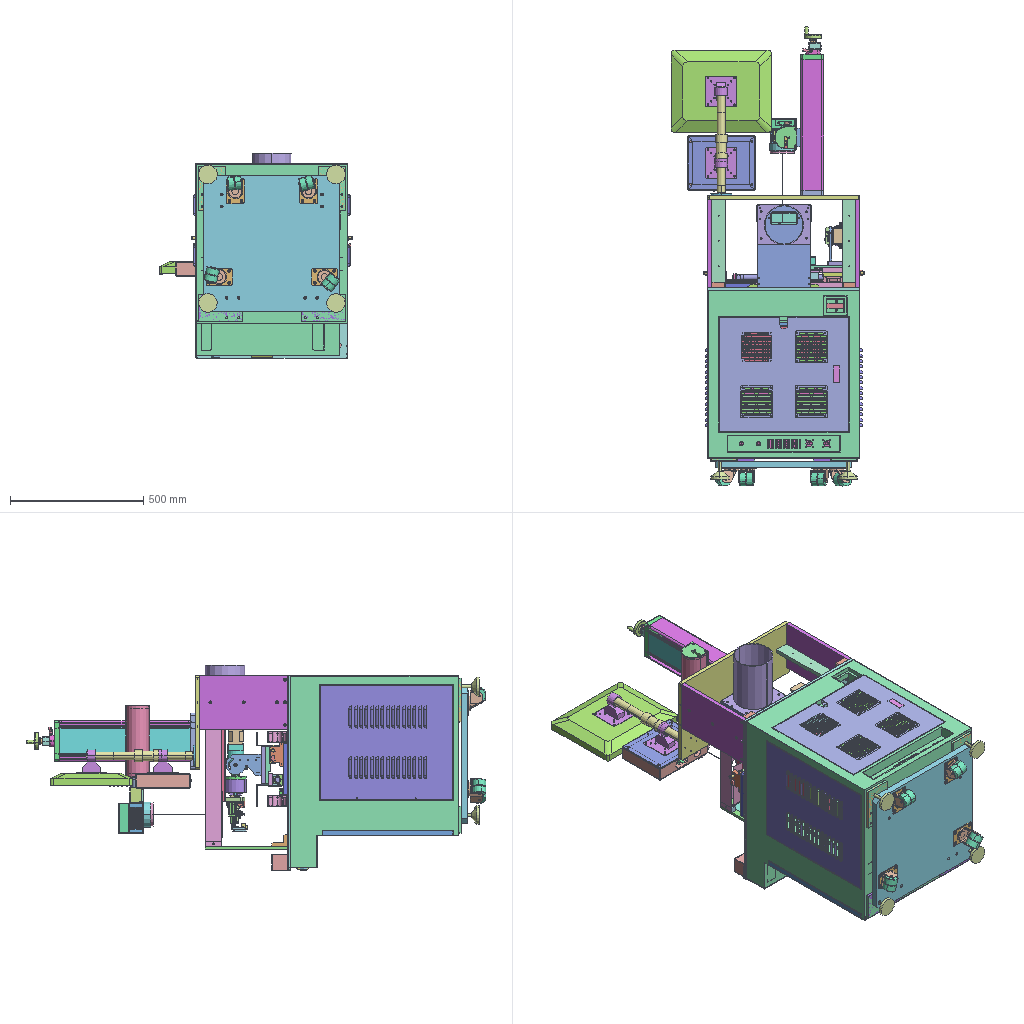Assembly | SolidWorks | 163 different items | 267 placed | box 725 x 1724 x 772 mm
Parts list (item | name | quantity | parent item | size | volume | features):
1 | (subassembly) | x1 | - | 570 x 345 x 350 mm | 5578892 mm3 | -
2 | (subassembly) | x1 | - | - | 5934131 mm3 | -
3 | (subassembly) | x1 | in 11 | 466 x 51.75 x 328.5 mm | 398956 mm3 | -
4 | (subassembly) | x1 | in 2 | 158.2 x 110.899 x 376 mm | 1286706 mm3 | -
5 | (subassembly) | x1 | in 2 | 158.2 x 109.159 x 384 mm | 1286706 mm3 | -
6 | (subassembly) | x2 | in 10 | 25 x 25 x 105.5 mm | 28768 mm3 | -
7 | (subassembly) | x1 | in 2 | 408 x 43 x 43 mm | 151257 mm3 | -
8 | (subassembly) | x1 | in 9 | 88 x 90 x 368 mm | 672845 mm3 | features CompositeCurve 4
9 | (subassembly) | x1 | in 15 | 408.184 x 175.143 x 489.463 mm | 1754817 mm3 | -
10 | (subassembly) | x2 | in 4, 5 | 61 x 31.574 x 113.094 mm | 38562 mm3 | -
11 | (subassembly) | x1 | - | - | 2228095 mm3 | -
12 | (subassembly) | x4 | in 11 | 102.422 x 68 x 90.224 mm | 133824 mm3 | -
13 | (subassembly) | x2 | in 4, 5 | 75 x 65 x 85 mm | 73444 mm3 | -
14 | (subassembly) | x2 | in 4, 5 | 65 x 40 x 80 mm | 46046 mm3 | -
15 | (subassembly) | x1 | - | - | 4821432 mm3 | -
16 | (subassembly) | x1 | - | 544.678 x 375 x 163 mm | 5912410 mm3 | -
17 | (subassembly) | x1 | in 15 | - | 3066920 mm3 | -
18 | (subassembly) | x1 | in 17 | 36.5 x 61 x 13 mm | 5415 mm3 | -
19 | (subassembly) | x1 | in 9 | 175 x 175 x 390 mm | 804489 mm3 | features CompositeCurve 19
20 | (subassembly) | x1 | in 17 | 33 x 36 x 47 mm | 34395 mm3 | -
21 | (subassembly) | x1 | in 2 | 63 x 30 x 510 mm | 298717 mm3 | -
22 | (subassembly) | x2 | in 2 | 14 x 16.166 x 60 mm | 6201 mm3 | -
23 | (subassembly) | x1 | - | 260 x 690 x 310 mm | 1689497 mm3 | -
24 | - | x1 | in 8 | 86 x 60 x 46 mm | 87351 mm3 | features ICE 4, 3DProfileFeature 2, Fillet 2, HoleWzd 2, Extrusion 1
25 | - | x1 | in 17 | - | - | features RefSurface 3, BaseBody 1, HoleWzd 1, MoveFace 1
26 | - | x2 | in 4, 5 | 60 x 60 x 108 mm | 230664 mm3 | features ICE 7, Chamfer 2, HoleWzd 2, CirPattern 1, Extrusion 1
27 | - | x4 | in 10 | 24 x 30 x 10 mm | 1863 mm3 | features BaseBody 1
28 | - | x2 | in 7 | 26 x 38 x 43 mm | 5706 mm3 | features BaseBody 1
29 | - | x1 | in 7 | 382 x 25 x 25 mm | 58255 mm3 | features BaseBody 1
30 | - | x1 | in 7 | 66 x 40 x 40 mm | 76631 mm3 | features BaseBody 1
31 | - | x2 | in 7 | 8 x 30.022 x 26 mm | 2480 mm3 | features BaseBody 1
32 | - | x6 | in 2, 4, 5 | 26 x 27.2 x 13.7 mm | 1973 mm3 | features BaseBody 1
33 | - | x2 | in 4, 5 | 80 x 80 x 66 mm | 244059 mm3 | features ICE 4, CirPattern 2, Extrusion 1, HoleWzd 1
34 | - | x1 | in 19 | 114 x 96.3 x 42.5 mm | 105828 mm3 | features Cut 4, Fillet 4, 3DProfileFeature 3, HoleWzd 3, LPattern 3, MirrorPattern 2, Chamfer 1, Extrusion 1
35 | - | x1 | in 17 | 63.283 x 62.5 x 55 mm | 41893 mm3 | features BaseBody 1
36 | - | x2 | in 19 | 35 x 35 x 3 mm | 1719 mm3 | features Chamfer 1, Extrusion 1
37 | - | x2 | in 14 | 65 x 40 x 17 mm | 37212 mm3 | features ICE 4, HoleWzd 3, Chamfer 1, Extrusion 1
38 | - | x2 | in 14 | 72.5 x 12 x 12 mm | 4576 mm3 | features Chamfer 2, ICE 2, Extrusion 1, HoleWzd 1
39 | - | x2 | in 14 | 8 x 8 x 67.5 mm | 2083 mm3 | features Chamfer 1, Fillet 1, Revolution 1
40 | - | x2 | in 14 | 8 x 8 x 68 mm | 2175 mm3 | features ICE 2, Chamfer 1, Extrusion 1, Fillet 1, HoleWzd 1
41 | - | x1 | in 17 | 44 x 53.969 x 18 mm | 32312 mm3 | features ICE 4, HoleWzd 2, Chamfer 1, CirPattern 1, Extrusion 1
42 | - | x1 | in 19 | 67 x 46.3 x 2 mm | 6002 mm3 | features 3DProfileFeature 1, Extrusion 1, Fillet 1, HoleWzd 1, LPattern 1
43 | - | x1 | in 19 | 114 x 96.5 x 58.3 mm | 315384 mm3 | features 3DProfileFeature 13, HoleWzd 13, Cut 10, Fillet 10, LPattern 9, SketchHole 7, Chamfer 3, MirrorPattern 3, Boss 2, VarFillet 2, Extrusion 1, RefAxis 1, RevCut 1
44 | - | x1 | in 19 | 175 x 175 x 309.5 mm | 221478 mm3 | features ICE 8, Draft 3, Chamfer 2, Extrusion 1, RevCut 1
45 | - | x1 | in 11 | 70 x 12 x 20 mm | 16291 mm3 | features Extrusion 1, HoleWzd 1
46 | - | x2 | in 17 | 8 x 28 x 28 mm | 2976 mm3 | features BaseBody 1
47 | - | x2 | in 19 | 75 x 35 x 6 mm | 9439 mm3 | features Fillet 9, Cut 1, Extrusion 1, LPattern 1
48 | - | x2 | in 16 | 115 x 89.5 x 115 mm | 126511 mm3 | features ICE 5, Chamfer 1, Extrusion 1, Fillet 1
49 | - | x1 | in 16 | 400 x 44 x 44 mm | 176887 mm3 | features ICE 1, Revolution 1
50 | - | x2 | in 6 | 25 x 25 x 85 mm | 25696 mm3 | features BaseBody 1
51 | - | x2 | in 6 | 12 x 12 x 80 mm | 3071 mm3 | features BaseBody 1
52 | - | x1 | in 19 | 38 x 38 x 76.09 mm | 37798 mm3 | features Boss 6, Chamfer 2, 3DProfileFeature 1, Cut 1, Extrusion 1, HoleWzd 1
53 | - | x1 | in 19 | 38 x 38 x 65.82 mm | 37638 mm3 | features Boss 6, Chamfer 2, 3DProfileFeature 1, Cut 1, Extrusion 1, HoleWzd 1
54 | - | x1 | in 11 | - | - | features RefSurface 1
55 | - | x2 | in 4, 5 | 57 x 57 x 77 mm | 166104 mm3 | features ICE 5, CirPattern 1, Extrusion 1, Fillet 1
56 | - | x4 | in 12 | 58 x 70 x 55 mm | 26099 mm3 | features ICE 7, Extrusion 1, Fillet 1
57 | - | x1 | in 8 | 55 x 30 x 12 mm | 13823 mm3 | features 3DProfileFeature 2, HoleWzd 2, Extrusion 1
58 | - | x8 | in 12 | 50 x 50 x 24 mm | 45851 mm3 | features Extrusion 1, Fillet 1, ICE 1
59 | - | x4 | in 12 | - | - | features ICE 2, ExtruRefSurface 1, Extrusion 1, Fillet 1
60 | - | x1 | in 16 | 200.4 x 34 x 181.25 mm | 892134 mm3 | features ICE 6, Cut 2, Fillet 2, Extrusion 1
61 | - | x2 | - | 25 x 42 x 25 mm | 13481 mm3 | features ICE 2, Chamfer 1, Extrusion 1
62 | - | x1 | in 19 | 95 x 33 x 95 mm | 58044 mm3 | features Chamfer 1, Revolution 1
63 | - | x2 | in 11 | 23 x 10 x 63 mm | 14490 mm3 | features Extrusion 1
64 | - | x3 | in 11 | 120 x 30 x 120 mm | 191392 mm3 | features ICE 3, Extrusion 1, Fillet 1
65 | - | x1 | in 8 | 40 x 34 x 6 mm | 5024 mm3 | features 3DProfileFeature 2, HoleWzd 2, Chamfer 1, Extrusion 1, ICE 1
66 | - | x1 | in 8 | 70 x 70 x 122 mm | 138507 mm3 | features ICE 10, 3DProfileFeature 2, HoleWzd 2, Extrusion 1
67 | - | x2 | in 3 | 10.262 x 51.5 x 305 mm | 30693 mm3 | features BaseBody 1
68 | - | x1 | in 3 | 69.588 x 27 x 29 mm | 10928 mm3 | features ICE 5, Chamfer 1, Extrusion 1
69 | - | x1 | in 3 | 78 x 45 x 15 mm | 24133 mm3 | features Fillet 3, ICE 2, Extrusion 1
70 | - | x1 | in 18 | 10 x 57.8 x 10 mm | 2265 mm3 | features RefAxis 3, 3DProfileFeature 1, ICE 1, RevCut 1, Revolution 1
71 | - | x1 | in 8 | 12 x 12 x 5 mm | 332.916 mm3 | features Chamfer 2, ICE 2, Extrusion 1
72 | - | x1 | in 18 | 36.5 x 25 x 13 mm | 3149 mm3 | features RefAxis 3, 3DProfileFeature 1, ICE 1, RevCut 1, Revolution 1
73 | - | x1 | in 16 | 375 x 307 x 47.5 mm | 4213214 mm3 | features BaseBody 1, ICE 1
74 | - | x1 | in 20 | 33 x 29 x 47 mm | 29608 mm3 | features ICE 6, RefAxis 6, RevCut 3, 3DProfileFeature 2, Revolution 2, Extrusion 1
75 | - | x1 | in 20 | 19.8 x 19.8 x 31 mm | 4724 mm3 | features RefAxis 9, 3DProfileFeature 3, RevCut 1, Revolution 1
76 | - | x2 | in 17 | 34 x 23.7 x 66.58 mm | 37160 mm3 | features BaseBody 1
77 | - | x2 | in 17 | 15 x 15 x 488 mm | 95639 mm3 | features BaseBody 1
78 | - | x1 | in 21 | 20 x 17.5 x 510 mm | 145503 mm3 | features BaseBody 1, HoleWzd 1, ICE 1, LPattern 1
79 | - | x2 | in 21 | 63 x 25.4 x 77.5 mm | 76607 mm3 | features BaseBody 1
80 | - | x2 | in 22 | 12 x 12 x 60 mm | 5613 mm3 | features BaseBody 1
81 | - | x2 | in 22 | 14 x 16.166 x 4 mm | 294.157 mm3 | features BaseBody 1
82 | - | x1 | in 8 | 84 x 77 x 265 mm | 79219 mm3 | features Extrusion 1, ICE 1
83 | - | x2 | in 22 | 14 x 16.166 x 4 mm | 294.157 mm3 | features BaseBody 1
84 | - | x1 | in 20 | 6 x 4 x 4 mm | 62.998 mm3 | features RefAxis 6, 3DProfileFeature 2, ICE 2, DelFace 1, Revolution 1
85 | - | x1 | in 9 | 46 x 46 x 247 mm | 277485 mm3 | features ICE 3, Chamfer 1, Extrusion 1
86 | - | x1 | in 16 | 250 x 200 x 3 mm | 149072 mm3 | features Cut 2, FlatPattern 1, HoleWzd 1, SMBaseFlange 1, SheetMetal 1
87 | - | x1 | in 16 | 254 x 204 x 52 mm | 161787 mm3 | features Cut 3, EdgeFlange 2, FlatPattern 1, ICE 1, SMBaseFlange 1, SheetMetal 1
88 | - | x1 | in 23 | 470 x 203 x 60 mm | 207704 mm3 | features HoleWzd 2, Cut 1, EdgeFlange 1, Fillet 1, FlatPattern 1, SMBaseFlange 1, SheetMetal 1
89 | - | x1 | in 23 | 169 x 5 x 279 mm | 235030 mm3 | features Chamfer 1, Extrusion 1, HoleWzd 1
90 | - | x2 | in 23 | 45 x 15 x 60 mm | 18806 mm3 | features HoleWzd 2, Chamfer 1, Extrusion 1
91 | - | x1 | in 23 | 150 x 200 x 200 mm | 202366 mm3 | features Extrusion 1, Fillet 1, HoleWzd 1, ICE 1
92 | - | x1 | in 23 | 200 x 10 x 310 mm | 193260 mm3 | features HoleWzd 3, Cut 2, Fillet 2, Extrusion 1
93 | - | x1 | in 8 | 36 x 33.5 x 4.5 mm | 1492 mm3 | features ICE 3, Extrusion 1
94 | - | x1 | in 23 | 130 x 50 x 300 mm | 125628 mm3 | features ICE 4, Cut 1, Fillet 1, MirrorPattern 1, Shell 1
95 | - | x2 | - | 80 x 60 x 60 mm | 26373 mm3 | features ICE 4, Fillet 3, Cut 1, Extrusion 1, MirrorPattern 1, Shell 1
96 | - | x1 | in 1 | 570 x 15 x 350 mm | 2765655 mm3 | features HoleWzd 4, Chamfer 2, Cut 1, Extrusion 1, Fillet 1
97 | - | x2 | in 1 | 200 x 15 x 330 mm | 982971 mm3 | features HoleWzd 3, Extrusion 1
98 | - | x2 | in 1 | 310 x 15 x 50 mm | 230397 mm3 | features HoleWzd 4, Extrusion 1
99 | - | x2 | in 1 | 50 x 20 x 200 mm | 193251 mm3 | features HoleWzd 3, Chamfer 1, Extrusion 1
100 | - | x4 | in 23 | 60 x 20 x 20 mm | 22148 mm3 | features HoleWzd 2, Extrusion 1
101 | - | x2 | in 4, 5 | 65 x 65 x 11 mm | 33278 mm3 | features HoleWzd 5, ICE 4, Chamfer 1, Extrusion 1, MirrorPattern 1
102 | - | x1 | in 11 | 570 x 10 x 730 mm | 4046206 mm3 | features HoleWzd 11, Cut 2, Chamfer 1, Extrusion 1, Fillet 1, ICE 1, LPattern 1
103 | - | x2 | in 2 | 20 x 60 x 14 mm | 8141 mm3 | features ICE 2, Extrusion 1, Fillet 1
104 | - | x1 | in 8 | 88 x 10 x 250 mm | 210737 mm3 | features ICE 5, 3DProfileFeature 2, HoleWzd 2, Extrusion 1
105 | - | x1 | in 11 | 510 x 25 x 510 mm | 6443430 mm3 | features HoleWzd 4, Chamfer 1, Extrusion 1
106 | - | x2 | in 4, 5 | 150 x 100 x 15 mm | 215343 mm3 | features HoleWzd 3, Chamfer 1, Cut 1, Extrusion 1
107 | - | x1 | in 2 | 200 x 570 x 15 mm | 1695675 mm3 | features HoleWzd 8, Chamfer 1, Extrusion 1
108 | - | x2 | in 2 | 80 x 25 x 70 mm | 122511 mm3 | features HoleWzd 3, Chamfer 1, Cut 1, Extrusion 1
109 | - | x1 | in 2 | 45 x 17 x 70 mm | 40738 mm3 | features HoleWzd 3, Cut 1, Extrusion 1
110 | - | x1 | in 2 | 150 x 20 x 330 mm | 769710 mm3 | features HoleWzd 5, Cut 3, Chamfer 1, Extrusion 1
111 | - | x2 | in 2 | 15 x 90 x 48 mm | 45379 mm3 | features HoleWzd 2, Chamfer 1, Cut 1, Extrusion 1, MirrorPattern 1
112 | - | x1 | in 2 | 20 x 49 x 30 mm | 2731 mm3 | features Chamfer 2, Cut 2, Fillet 1, FlatPattern 1, SMBaseFlange 1, SheetMetal 1
113 | - | x2 | in 2 | 100 x 20 x 3 mm | 5311 mm3 | features Chamfer 1, Cut 1, FlatPattern 1, HoleWzd 1, SMBaseFlange 1, SheetMetal 1
114 | - | x1 | in 2 | 130 x 31.5 x 40 mm | 9150 mm3 | features Chamfer 1, Cut 1, FlatPattern 1, SMBaseFlange 1, SheetMetal 1
115 | - | x4 | in 11 | 70 x 180 x 70 mm | 90530 mm3 | features Chamfer 1, Extrusion 1, ICE 1
116 | - | x1 | in 2 | 18 x 25 x 18 mm | 6362 mm3 | features Extrusion 1
117 | - | x1 | in 2 | 100 x 31.5 x 40 mm | 7350 mm3 | features Chamfer 1, Cut 1, FlatPattern 1, SMBaseFlange 1, SheetMetal 1
118 | - | x2 | in 13 | 8 x 18 x 28 mm | 3206 mm3 | features HoleWzd 3, Chamfer 1, Extrusion 1, ICE 1
119 | - | x1 | in 3 | 110 x 16.5 x 143 mm | 24337 mm3 | features Extrusion 1, Fillet 1, ICE 1
120 | - | x1 | in 11 | 570 x 640 x 720 mm | 3281506 mm3 | features ICE 78, HoleWzd 16, 3DProfileFeature 7, Fillet 5, Cut 3, LPattern 2, MoveFace 2, Chamfer 1, Extrusion 1, MirrorPattern 1
121 | - | x1 | in 11 | 190 x 70 x 1.5 mm | 17641 mm3 | features Extrusion 1, Fillet 1, HoleWzd 1, ICE 1
122 | - | x2 | in 11 | 430 x 500 x 30.5 mm | 310221 mm3 | features ICE 10, LPattern 4, MirrorPattern 3, HoleWzd 2, 3DProfileFeature 1, Chamfer 1, Extrusion 1, Fillet 1, Revolution 1, Shell 1
123 | - | x1 | in 11 | 485 x 450 x 20 mm | 237812 mm3 | features ICE 14, LPattern 4, Chamfer 3, Fillet 2, MirrorPattern 2, Extrusion 1, Shell 1
124 | - | x4 | in 11 | 40 x 40 x 420 mm | 49080 mm3 | features ICE 3, Cut 2, 3DProfileFeature 1, Extrusion 1, Fillet 1, HoleWzd 1
125 | - | x1 | in 11 | 510 x 13 x 298 mm | 241231 mm3 | features ICE 3, Fillet 2, LPattern 2, Extrusion 1, HoleWzd 1, MoveFace 1, Revolution 1
126 | - | x2 | - | 76 x 40 x 418 mm | 200180 mm3 | features Fillet 2, ICE 2, Sweep 1, SweepCut 1
127 | - | x1 | in 11 | 570 x 510 x 20 mm | 346646 mm3 | features ICE 4, Extrusion 1, Shell 1
128 | - | x1 | in 3 | 429 x 30.5 x 260 mm | 225455 mm3 | features ICE 19, LPattern 2, Extrusion 1, Fillet 1
129 | - | x1 | in 3 | 466 x 50 x 19 mm | 83409 mm3 | features ICE 4, Extrusion 1, Shell 1
130 | - | x2 | in 11 | 100 x 10 x 165 mm | 162650 mm3 | features HoleWzd 3, 3DProfileFeature 2, Chamfer 1, Extrusion 1
131 | - | x2 | in 11 | 165 x 10 x 100 mm | 162650 mm3 | features HoleWzd 2, Chamfer 1, Extrusion 1
132 | - | x1 | in 11 | 445 x 460 x 105 mm | 15966667 mm3 | features ICE 9, HoleWzd 5, MoveFace 2, Extrusion 1, Fillet 1, LPattern 1, Shell 1
133 | - | x1 | in 11 | 90 x 1.5 x 20 mm | 2636 mm3 | features Extrusion 1, Fillet 1, ICE 1
134 | - | x1 | in 16 | 40 x 80 x 80 mm | 66296 mm3 | features HoleWzd 2, Chamfer 1, CirPattern 1, ICE 1, Revolution 1
135 | - | x2 | in 13 | 75 x 65 x 15 mm | 61686 mm3 | features HoleWzd 4, Chamfer 1, Cut 1, Extrusion 1, Fillet 1, ICE 1
136 | - | x6 | in 13 | 30 x 8 x 8 mm | 1396 mm3 | features Chamfer 1, Extrusion 1, Fillet 1, ICE 1
137 | - | x1 | in 8 | 59.5 x 86 x 6 mm | 29999 mm3 | features ICE 2, Extrusion 1, Fillet 1
138 | - | x2 | in 13 | 62.5 x 10 x 10 mm | 4365 mm3 | features Chamfer 1, CirPattern 1, Extrusion 1, HoleWzd 1, ICE 1
139 | - | x2 | in 4, 5 | 80 x 80 x 53 mm | 69285 mm3 | features ICE 4, HoleWzd 3, Chamfer 1, CirPattern 1, Extrusion 1, Fillet 1
140 | - | x2 | in 4, 5 | 80 x 131 x 10 mm | 79591 mm3 | features HoleWzd 3, Cut 1, Extrusion 1, Fillet 1, ICE 1
141 | - | x2 | in 4, 5 | 80 x 131 x 10 mm | 79591 mm3 | features HoleWzd 3, Cut 1, Extrusion 1, Fillet 1, ICE 1
142 | - | x4 | in 4, 5 | 12 x 12 x 8 mm | 497 mm3 | features Chamfer 1, Extrusion 1
143 | - | x4 | in 4, 5 | 14 x 14 x 21.5 mm | 1140 mm3 | features ICE 4, Chamfer 1, Extrusion 1, Fillet 1
144 | - | x2 | in 4, 5 | 15 x 33.8 x 31.2 mm | 1093 mm3 | features EdgeFlange 2, FlatPattern 1, HoleWzd 1, SMBaseFlange 1, SheetMetal 1
145 | - | x4 | in 4, 5 | 30 x 22 x 2 mm | 1213 mm3 | features Cut 1, Fillet 1, FlatPattern 1, HoleWzd 1, SMBaseFlange 1, SheetMetal 1
146 | - | x2 | in 10 | 8 x 10 x 51 mm | 3618 mm3 | features HoleWzd 3, Chamfer 1, Extrusion 1
147 | - | x2 | in 10 | 15 x 15 x 16 mm | 1985 mm3 | features Chamfer 1, Extrusion 1, HoleWzd 1
148 | - | x1 | in 8 | 88 x 84 x 12 mm | 63664 mm3 | features ICE 6, 3DProfileFeature 3, HoleWzd 3, Extrusion 1
149 | - | x2 | in 10 | 28 x 10 x 2.5 mm | 464.649 mm3 | features Extrusion 1, Fillet 1, ICE 1
150 | - | x1 | in 23 | 200 x 310 x 10 mm | 568919 mm3 | features HoleWzd 4, Cut 1, Extrusion 1, Fillet 1
151 | - | x2 | in 23 | 15 x 45 x 50 mm | 15193 mm3 | features HoleWzd 2, Chamfer 1, Extrusion 1, Fillet 1, ICE 1
152 | - | x1 | in 17 | - | - | features RefSurface 8, HoleWzd 2, BaseBody 1
153 | - | x1 | in 17 | - | - | features RefSurface 5, HoleWzd 2, BaseBody 1, CirPattern 1, MirrorPattern 1, RefAxis 1
154 | - | x1 | in 17 | 18 x 585 x 18 mm | 134308 mm3 | features ICE 4, Chamfer 2, BaseBody 1, Fillet 1, HoleWzd 1
155 | - | x1 | in 17 | - | - | features RefSurface 6, BaseBody 1
156 | - | x1 | in 17 | - | - | features RefSurface 4, BaseBody 1
157 | - | x1 | in 17 | 210 x 20 x 85.5 mm | 334526 mm3 | features BaseBody 1
158 | - | x1 | in 17 | - | - | features RefSurface 4, BaseBody 1
159 | - | x1 | in 8 | 88 x 84 x 12 mm | 42695 mm3 | features ICE 6, 3DProfileFeature 3, HoleWzd 3, Extrusion 1, MoveFace 1
160 | ECY11-S3M-150 (subassembly) | x1 | - | - | - | -
161 | MAT9763-01-013T Cylinder Press Rod  | x1 | - | - | - | -
162 | MAT9763-01-015T Riser Block  | x1 | - | - | - | -
163 | MKB12-10LZ-M9B (subassembly) | x1 | - | - | - | -
Mates (type | each side: item.copy, entity, surface, feature), first 437 of 490 lines:
In the top assembly
Coincident | 102.1 face plane Boss-Extrude 1 | assembly face | 3 times
DistanceDim | assembly face | 102.1 face plane Boss-Extrude 1
Coincident | 102.1 face plane Boss-Extrude 1 | 107.1 face plane Boss-Extrude 1
Coincident | 102.1 face plane Boss-Extrude 1 | 126.1 face plane Sweep 1
Parallel | 102.1 face plane Boss-Extrude 1 | assembly face
Width | assembly face | assembly face | 102.1 face plane Boss-Extrude 1 | 102.1 face plane Boss-Extrude 1
DistanceDim | 150.1 face plane Boss-Extrude 1 | 102.1 face plane Boss-Extrude 1
DistanceDim | 107.1 face plane Boss-Extrude 1 | 102.1 face plane Boss-Extrude 1
Width | 107.1 face plane Boss-Extrude 1 | 107.1 face plane Boss-Extrude 1 | 102.1 face plane Boss-Extrude 1 | 102.1 face plane Boss-Extrude 1
Coincident | 102.1 face plane Boss-Extrude 1 | 95.1 face plane Boss-Extrude 1 | 2 times
Coincident | 102.1 face plane Boss-Extrude 1 | 95.2 face plane Boss-Extrude 1 | 2 times
Width | 92.1 face plane Boss-Extrude 1 | 92.1 face plane Boss-Extrude 1 | 102.1 face plane Boss-Extrude 1 | 102.1 face plane Boss-Extrude 1
Width | 97.1 face plane Boss-Extrude 1 | 97.2 face plane Boss-Extrude 1 | 120.1 face plane Boss-Extrude 1 | 120.1 face plane Boss-Extrude 1
Coincident | 102.1 face plane Boss-Extrude 1 | 99.1 face plane Boss-Extrude 1 | 2 times
Coincident | 157.1 face plane Import 1 | 96.1 face plane Boss-Extrude 1 | 2 times
Coincident | 134.1 face plane Revolve 1 | 96.1 face plane Boss-Extrude 1
DistanceDim | 134.1 plane | 96.1 face plane Boss-Extrude 1 | 2 times
Coincident | 102.1 face plane Boss-Extrude 1 | 95.1 face plane Boss-Extrude 3
Coincident | 102.1 face plane Boss-Extrude 1 | 95.2 face plane Boss-Extrude 4
Concentric | 95.2 face cylinder Cut-Extrude 4 | 61.1 face cylinder Boss-Extrude 1
Coincident | 95.2 face plane Boss-Extrude 1 | 61.1 face plane Boss-Extrude 3
Concentric | 61.2 face cylinder Boss-Extrude 1 | 95.1 face cylinder Cut-Extrude 4
Coincident | 61.2 face plane Boss-Extrude 3 | 95.1 face plane Boss-Extrude 1
DistanceDim | 157.1 face plane Import 1 | 96.1 face plane Boss-Extrude 1
Coincident | 102.1 face plane Boss-Extrude 1 | 126.2 face plane Sweep 1
Coincident | 107.1 face plane Boss-Extrude 1 | 126.2 face plane Sweep 1
Coincident | 107.1 face plane Boss-Extrude 1 | 126.1 face plane Sweep 1
Coincident | 151.1 face plane Boss-Extrude 1 | 102.1 face plane Boss-Extrude 1
In subassembly 2
Parallel | 107.2 face plane Boss-Extrude 1 | 78.1 plane
Coincident | 79.1 face plane Import 1 | 108.1 face plane Cut-Extrude 1 | 2 times
Width | 108.1 face plane Boss-Extrude 1 | 108.1 face plane Boss-Extrude 1 | 79.1 face plane Import 1 | 79.1 face plane Import 1
Coincident | 79.2 face plane Import 1 | 108.2 face plane Cut-Extrude 1 | 2 times
Width | 108.2 face plane Boss-Extrude 1 | 108.2 face plane Boss-Extrude 1 | 79.2 face plane Import 1 | 79.2 face plane Import 1
Coincident | 110.1 face plane Boss-Extrude 1 | 108.2 face plane Boss-Extrude 1
Width | 78.1 face plane Import 1 | 78.1 face plane Boss-Extrude 1 | 107.2 face plane Boss-Extrude 1 | 107.2 face plane Boss-Extrude 1
Coincident | 106.1 face plane Boss-Extrude 1 | 110.1 face plane Boss-Extrude 1 | 2 times
Width | 106.1 face plane Boss-Extrude 1 | 106.1 face plane Boss-Extrude 1 | 110.1 face plane Boss-Extrude 1 | 110.1 face plane Boss-Extrude 1
Coincident | 106.2 face plane Boss-Extrude 1 | 110.1 face plane Boss-Extrude 1 | 2 times
Width | 110.1 face plane Boss-Extrude 1 | 110.1 face plane Boss-Extrude 1 | 106.2 face plane Boss-Extrude 1 | 106.2 face plane Boss-Extrude 1
Coincident | 107.2 face plane Boss-Extrude 1 | 111.1 face plane Boss-Extrude 1 | 2 times
Width | 108.1 face plane Boss-Extrude 1 | 108.2 face plane Boss-Extrude 1 | 110.1 face plane Boss-Extrude 1 | 110.1 face plane Boss-Extrude 1
Coincident | 107.2 face plane Boss-Extrude 1 | 28.1 face plane Import 1
Coincident | 110.1 face plane Boss-Extrude 1 | 30.1 face plane Import 1
Width | 28.1 face plane Import 1 | 28.2 face plane Import 1 | 107.2 face plane Boss-Extrude 1 | 107.2 face plane Boss-Extrude 1
Width | 30.1 face plane Import 1 | 30.1 face plane Import 1 | 110.1 face plane Boss-Extrude 1 | 110.1 face plane Boss-Extrude 1
Coincident | 108.1 face plane Boss-Extrude 1 | 110.1 face plane Cut-Extrude 1
Width | 108.1 face plane Boss-Extrude 1 | 108.1 face plane Boss-Extrude 1 | 111.1 face plane Boss-Extrude 1 | 111.1 face plane Boss-Extrude 1
Coincident | 107.2 face plane Boss-Extrude 1 | 78.1 face plane Import 1
Concentric | 111.1 face cylinder M12x1.25 Tapped Hole 2 | 80.1 face cylinder Import 1
Coincident | 111.1 face plane Boss-Extrude 1 | 81.1 face plane Import 1
Coincident | 107.2 face plane Boss-Extrude 1 | 111.2 face plane Boss-Extrude 1 | 2 times
Width | 108.2 face plane Boss-Extrude 1 | 108.2 face plane Boss-Extrude 1 | 111.2 face plane Boss-Extrude 1 | 111.2 face plane Boss-Extrude 1
Concentric | 111.2 face cylinder M12x1.25 Tapped Hole 2 | 80.2 face cylinder Import 1
Coincident | 111.2 face plane Boss-Extrude 1 | 81.2 face plane Import 1
Concentric | 111.1 face cylinder M12x1.25 Tapped Hole 2 | 103.1 face cylinder Cut-Extrude 1
Concentric | 111.2 face cylinder M12x1.25 Tapped Hole 2 | 103.2 face cylinder Cut-Extrude 1
Coincident | 111.2 face plane Boss-Extrude 1 | 103.2 face plane Cut-Extrude 1
Coincident | 111.1 face plane Boss-Extrude 1 | 103.1 face plane Cut-Extrude 1
Width | 109.1 face plane Boss-Extrude 1 | 109.1 face plane Boss-Extrude 1 | 30.1 face plane Import 1 | 30.1 face plane Import 1
Width | 30.1 face plane Import 1 | 30.1 face plane Import 1 | 109.1 face plane Boss-Extrude 1 | 109.1 face plane Boss-Extrude 1
Coincident | 30.1 face plane Import 1 | 109.1 face plane Cut-Extrude 1
DistanceDim | 110.1 face plane Boss-Extrude 1 | 107.2 face plane Boss-Extrude 1
Width | 112.1 face plane Base-Flange 1 | 112.1 face plane Base-Flange 1 | 109.1 face plane Boss-Extrude 1 | 109.1 face plane Boss-Extrude 1
Coincident | 109.1 face plane Boss-Extrude 1 | 112.1 face plane Base-Flange 1 | 2 times
Coincident | 107.2 face plane Boss-Extrude 1 | 113.1 face plane Base-Flange 1 | 2 times
Parallel | 107.2 face plane Boss-Extrude 1 | 113.1 face plane Base-Flange 1
Coincident | 32.1 face plane Import 1 | 113.1 face plane Base-Flange 1
Width | 32.1 face plane Import 1 | 32.1 face plane Import 1 | 113.1 face plane Base-Flange 1 | 113.1 face plane Base-Flange 1 | 2 times
DistanceDim | 113.1 face plane Base-Flange 1 | 107.2 face plane Boss-Extrude 1
Coincident | 107.2 face plane Boss-Extrude 1 | 113.2 face plane Base-Flange 1 | 2 times
DistanceDim | 113.2 face plane Base-Flange 1 | 107.2 face plane Boss-Extrude 1
Coincident | 32.2 face plane Import 1 | 113.2 face plane Base-Flange 1
Width | 32.2 face plane Import 1 | 32.2 face plane Import 1 | 113.2 face plane Base-Flange 1 | 113.2 face plane Base-Flange 1 | 2 times
Concentric | 109.1 face cylinder Ø18.0 (18) DiameterHole 1 | 116.1 face cylinder Boss-Extrude 1
Coincident | 30.1 face plane Import 1 | 116.1 face plane Boss-Extrude 1
Coincident | 110.1 face plane Boss-Extrude 1 | 117.1 face plane Base-Flange 1 | 2 times
Width | 106.1 face plane Boss-Extrude 1 | 106.2 face plane Boss-Extrude 1 | 117.1 face plane Base-Flange 1 | 117.1 face plane Base-Flange 1
Coincident | 110.1 face plane Boss-Extrude 1 | 114.1 face plane Base-Flange 1 | 2 times
Coincident | 106.1 face plane Boss-Extrude 1 | 114.1 face plane Base-Flange 1
In subassembly 5
Concentric | 26.1 face cylinder Cut-Extrude 1 | 55.1 face cylinder Boss-Extrude 3
Coincident | 26.1 face plane Boss-Extrude 1 | 55.1 face plane Boss-Extrude 1
Concentric | 26.1 face cylinder CirPattern 1 | 55.1 face cylinder Cut-Extrude 2
Concentric | 26.1 face cylinder Boss-Extrude 2 | 101.1 face cylinder Cut-Extrude 2
Coincident | 26.1 face plane Boss-Extrude 2 | 101.1 face plane Boss-Extrude 1
Parallel | 26.1 face plane Boss-Extrude 1 | 101.1 face plane Boss-Extrude 1
Concentric | 26.1 face cylinder Boss-Extrude 5 | 33.1 face cylinder Boss-Extrude 1
Concentric | 33.1 face cylinder Boss-Extrude 1 | 138.1 face cylinder Boss-Extrude 1
Concentric | 26.1 face cylinder Boss-Extrude 5 | 139.1 face cylinder Boss-Extrude 1
Coincident | 26.1 face plane Boss-Extrude 4 | 139.1 face plane Boss-Extrude 1
Coincident | 33.1 face plane Boss-Extrude 1 | 139.1 face plane Boss-Extrude 2
Concentric | 33.1 face cylinder CirPattern 2 | 139.1 face cylinder CirPattern 1
Coincident | 101.1 face plane Boss-Extrude 1 | 140.1 face plane Boss-Extrude 1
Concentric | 101.1 face cylinder M6 Tapped Hole 1 | 140.1 face cylinder Hole 1
Concentric | 140.1 face cylinder Hole 1 | 142.1 face cylinder Boss-Extrude 1
Concentric | 143.1 face cylinder Boss-Extrude 2 | 142.1 face cylinder Boss-Extrude 1
Coincident | 140.1 face plane Boss-Extrude 1 | 142.1 face plane Boss-Extrude 1
Concentric | 141.1 face cylinder Hole 1 | 142.2 face cylinder Boss-Extrude 1
Coincident | 141.1 face plane Hole 1 | 142.2 face plane Boss-Extrude 1
Concentric | 142.2 face cylinder Boss-Extrude 1 | 143.2 face cylinder Boss-Extrude 2
Coincident | 101.1 face plane Boss-Extrude 1 | 141.1 face plane Boss-Extrude 1
Coincident | 101.1 face plane Boss-Extrude 1 | 143.2 face plane Boss-Extrude 2
Coincident | 101.1 face plane Boss-Extrude 1 | 143.1 face plane Boss-Extrude 2
Parallel | 26.1 face plane Boss-Extrude 1 | 140.1 face plane Cut-Extrude 4
Coincident | 140.1 face plane Boss-Extrude 1 | 106.3 face plane Boss-Extrude 1
Coincident | 135.1 face plane Boss-Extrude 1 | 37.1 face plane Boss-Extrude 1
Concentric | 136.1 face cylinder Boss-Extrude 2 | 37.1 face cylinder Ø8.0 (8) DiameterHole 1
Concentric | 136.2 face cylinder Boss-Extrude 2 | 37.1 face cylinder Ø8.0 (8) DiameterHole 1
Coincident | 135.1 face plane Boss-Extrude 1 | 50.1 face plane Import 1
Parallel | 5.1 face | 37.1 face plane Boss-Extrude 1
Concentric | 140.1 face cylinder M6 Tapped Hole 1 | 106.3 face cylinder M6 Hex Socket Screw Counterbore Hole 1
Concentric | 106.3 face cylinder M6 Hex Socket Screw Counterbore Hole 1 | 141.1 face cylinder M6 Tapped Hole 1
Coincident | 106.3 face plane Boss-Extrude 1 | 141.1 face plane Boss-Extrude 1
Concentric | 135.1 face cylinder M4 Hex Socket Screw Counterbore Hole 1 | 50.1 face cylinder Import 1 | 2 times
Coincident | 139.1 face plane Cut-Extrude 3 | 144.1 face plane Base-Flange 1
Coincident | 101.1 face plane Boss-Extrude 1 | 145.1 face plane Base-Flange 1 | 2 times
Width | 145.1 face plane Base-Flange 1 | 145.1 face plane Base-Flange 1 | 101.1 face plane Boss-Extrude 1 | 101.1 face plane Boss-Extrude 1
Coincident | 145.1 face plane Base-Flange 1 | 32.2 face plane Import 1
DistanceDim | 32.2 face plane Import 1 | 145.1 face plane Base-Flange 1
Width | 32.2 face plane Import 1 | 32.2 face plane Import 1 | 145.1 face plane Base-Flange 1 | 145.1 face plane Base-Flange 1
Coincident | 101.1 face plane Boss-Extrude 1 | 145.2 face plane Base-Flange 1 | 2 times
Width | 101.1 face plane Cut-Extrude 3 | 101.1 face plane Mirror 1 | 145.2 face plane Base-Flange 1 | 145.2 face plane Base-Flange 1
DistanceDim | 32.1 face plane Import 1 | 145.2 face plane Base-Flange 1
Width | 32.1 face plane Import 1 | 32.1 face plane Import 1 | 145.2 face plane Base-Flange 1 | 145.2 face plane Base-Flange 1
Concentric | 139.1 face cylinder M4 Tapped Hole 2 | 144.1 face cylinder Ø4.5 (4.5) DiameterHole 1 | 2 times
DistanceDim | 33.1 face plane CirPattern 1 | 118.1 face plane Boss-Extrude 1
Parallel | 135.1 face plane Boss-Extrude 1 | 33.1 face plane Boss-Extrude 2
In subassembly 13
Coincident | 135.2 face plane Hole 1 | 138.2 face plane Boss-Extrude 1
Concentric | 135.2 face cylinder Ø8.0 (8) DiameterHole 1 | 136.3 face cylinder Boss-Extrude 1
Coincident | 135.2 face plane Boss-Extrude 1 | 136.3 face plane Boss-Extrude 1
Concentric | 135.2 face cylinder Ø8.0 (8) DiameterHole 1 | 136.4 face cylinder Boss-Extrude 1
Coincident | 135.2 face plane Boss-Extrude 1 | 136.4 face plane Boss-Extrude 1
Concentric | 135.2 face cylinder Ø8.0 (8) DiameterHole 1 | 136.5 face cylinder Boss-Extrude 1
Coincident | 135.2 face plane Boss-Extrude 1 | 136.5 face plane Boss-Extrude 1
Concentric | 135.2 face cylinder Hole 1 | 138.2 face cylinder Boss-Extrude 1
Concentric | 138.2 face cylinder Boss-Extrude 1 | 118.2 face cylinder Cut-Extrude 1
Coincident | 135.2 face plane Boss-Extrude 1 | 118.2 face plane Boss-Extrude 1
Concentric | 135.2 face cylinder Hole 1 | 118.2 face cylinder M4 Tapped Hole 2
Parallel | 135.2 face plane Boss-Extrude 1 | 138.2 face plane CirPattern 1
In subassembly 14
Concentric | 37.2 face cylinder Cut-Extrude 1 | 38.1 face cylinder Boss-Extrude 1
Coincident | 37.2 face plane Cut-Extrude 1 | 38.1 face plane Boss-Extrude 1
Concentric | 37.2 face cylinder Ø6.0 (6) DiameterHole 1 | 39.1 face cylinder Revolve 1
Coincident | 37.2 face plane Boss-Extrude 1 | 39.1 face plane Revolve 1
Coincident | 37.2 face plane Cut-Extrude 2 | 40.1 face plane Boss-Extrude 1
Tangent | 37.2 face plane Cut-Extrude 2 | 40.1 face cylinder Boss-Extrude 1
In subassembly 10
Coincident | 51.1 face plane Import 1 | 149.1 face plane Boss-Extrude 1
Coincident | 51.1 face plane Import 1 | 149.1 face plane Cut-Extrude 1 | 2 times
Coincident | 146.1 face plane Boss-Extrude 1 | 149.1 face plane Boss-Extrude 1
Concentric | 51.1 face cylinder Import 1 | 146.1 face cylinder Hole Size per Hexagon Socket Head Cap Screw Type 1
Parallel | 146.1 face plane Boss-Extrude 1 | 149.1 face plane Boss-Extrude 1
Concentric | 146.1 face cylinder M4 Tapped Hole 1 | 147.1 face cylinder Boss-Extrude 1
Coincident | 146.1 face plane Boss-Extrude 1 | 147.1 face plane Boss-Extrude 1
Concentric | 50.2 face cylinder Import 1 | 27.1 face cylinder Import 1
Concentric | 50.2 face cylinder Import 1 | 27.2 face cylinder Import 1
Coincident | 50.2 face plane Import 1 | 27.2 face plane Import 1
Coincident | 50.2 face plane Import 1 | 27.1 face plane Import 1
Parallel | 50.2 face plane Import 1 | 146.1 face plane Boss-Extrude 1
In subassembly 6
DistanceDim | 51.2 face plane Import 1 | 50.3 face plane Import 1
Concentric | 50.3 face cylinder Import 1 | 51.2 face cylinder Import 1
In subassembly 21
Coincident | 79.3 face plane Import 1 | 78.2 face plane Import 1
Width | 79.3 face plane Import 1 | 79.3 face plane Import 1 | 78.2 face plane Import 1 | 78.2 face plane Import 1
LimitDistanceDim | 78.2 face plane Boss-Extrude 1 | 79.3 face plane Import 1
Coincident | 78.2 face plane Import 1 | 79.4 face plane Import 1
Coincident | 79.3 face plane Import 1 | 79.4 face plane Import 1
DistanceDim | 79.3 face plane Import 1 | 79.4 face plane Import 1
In subassembly 4
Concentric | 26.1 face cylinder Cut-Extrude 1 | 55.1 face cylinder Boss-Extrude 3
Coincident | 26.1 face plane Boss-Extrude 1 | 55.1 face plane Boss-Extrude 1
Concentric | 26.1 face cylinder CirPattern 1 | 55.1 face cylinder Cut-Extrude 2
Concentric | 26.1 face cylinder Boss-Extrude 2 | 101.1 face cylinder Cut-Extrude 2
Coincident | 26.1 face plane Boss-Extrude 2 | 101.1 face plane Boss-Extrude 1
Parallel | 26.1 face plane Boss-Extrude 1 | 101.1 face plane Boss-Extrude 1
Concentric | 26.1 face cylinder Boss-Extrude 5 | 33.1 face cylinder Boss-Extrude 1
Concentric | 33.1 face cylinder Boss-Extrude 1 | 138.1 face cylinder Boss-Extrude 1
DistanceDim | 135.1 face plane Boss-Extrude 1 | 33.1 face plane Boss-Extrude 2
Concentric | 26.1 face cylinder Boss-Extrude 5 | 139.1 face cylinder Boss-Extrude 1
Coincident | 26.1 face plane Boss-Extrude 4 | 139.1 face plane Boss-Extrude 1
Coincident | 33.1 face plane Boss-Extrude 1 | 139.1 face plane Boss-Extrude 2
Concentric | 33.1 face cylinder CirPattern 2 | 139.1 face cylinder CirPattern 1
Coincident | 101.1 face plane Boss-Extrude 1 | 140.1 face plane Boss-Extrude 1
Concentric | 101.1 face cylinder M6 Tapped Hole 1 | 140.1 face cylinder Hole 1
Concentric | 140.1 face cylinder Hole 1 | 142.1 face cylinder Boss-Extrude 1
Concentric | 143.1 face cylinder Boss-Extrude 2 | 142.1 face cylinder Boss-Extrude 1
Coincident | 140.1 face plane Boss-Extrude 1 | 142.1 face plane Boss-Extrude 1
Concentric | 141.1 face cylinder Hole 1 | 142.2 face cylinder Boss-Extrude 1
Coincident | 141.1 face plane Hole 1 | 142.2 face plane Boss-Extrude 1
Concentric | 142.2 face cylinder Boss-Extrude 1 | 143.2 face cylinder Boss-Extrude 2
Coincident | 101.1 face plane Boss-Extrude 1 | 141.1 face plane Boss-Extrude 1
Coincident | 139.1 face plane Cut-Extrude 3 | 144.1 face plane Base-Flange 1
Concentric | 139.1 face cylinder M4 Tapped Hole 2 | 144.1 face cylinder Ø4.5 (4.5) DiameterHole 1 | 2 times
Parallel | 26.1 face plane Boss-Extrude 6 | 139.1 face plane Cut-Extrude 4
Coincident | 101.1 face plane Boss-Extrude 1 | 143.2 face plane Boss-Extrude 2
Coincident | 101.1 face plane Boss-Extrude 1 | 143.1 face plane Boss-Extrude 2
Parallel | 26.1 face plane Boss-Extrude 1 | 140.1 face plane Cut-Extrude 4
Coincident | 140.1 face plane Boss-Extrude 1 | 106.3 face plane Boss-Extrude 1
Coincident | 135.1 face plane Boss-Extrude 1 | 37.1 face plane Boss-Extrude 1
Concentric | 136.1 face cylinder Boss-Extrude 2 | 37.1 face cylinder Ø8.0 (8) DiameterHole 1
Concentric | 136.2 face cylinder Boss-Extrude 2 | 37.1 face cylinder Ø8.0 (8) DiameterHole 1
Coincident | 135.1 face plane Boss-Extrude 1 | 50.1 face plane Import 1
Parallel | 4.1 face | 37.1 face plane Boss-Extrude 1
Coincident | 135.1 face plane Boss-Extrude 1 | 4.1 face
Concentric | 135.1 face cylinder M4 Hex Socket Screw Counterbore Hole 1 | 4.1 face | 4 times
Concentric | 140.1 face cylinder M6 Tapped Hole 1 | 106.3 face cylinder M6 Hex Socket Screw Counterbore Hole 1
Concentric | 106.3 face cylinder M6 Hex Socket Screw Counterbore Hole 1 | 141.1 face cylinder M6 Tapped Hole 1
Coincident | 106.3 face plane Boss-Extrude 1 | 141.1 face plane Boss-Extrude 1
Concentric | 135.1 face cylinder M4 Hex Socket Screw Counterbore Hole 1 | 50.1 face cylinder Import 1 | 2 times
Coincident | 145.2 face plane Base-Flange 1 | 32.1 face plane Import 1
Width | 32.1 face plane Import 1 | 32.1 face plane Import 1 | 145.2 face plane Base-Flange 1 | 145.2 face plane Base-Flange 1
DistanceDim | 32.1 face plane Import 1 | 145.2 face plane Base-Flange 1
Coincident | 145.1 face plane Base-Flange 1 | 32.2 face plane Import 1
Width | 32.2 face plane Import 1 | 32.2 face plane Import 1 | 145.1 face plane Base-Flange 1 | 145.1 face plane Base-Flange 1
DistanceDim | 145.1 face plane Base-Flange 1 | 32.2 face plane Import 1
Coincident | 101.1 face plane Boss-Extrude 1 | 145.1 face plane Base-Flange 1
DistanceDim | 101.1 face plane Boss-Extrude 1 | 145.1 face plane Base-Flange 1
Width | 101.1 face plane Boss-Extrude 1 | 101.1 face plane Boss-Extrude 1 | 145.1 face plane Base-Flange 1 | 145.1 face plane Base-Flange 1
Coincident | 101.1 face plane Boss-Extrude 1 | 145.2 face plane Base-Flange 1
DistanceDim | 145.2 face plane Base-Flange 1 | 101.1 face plane Boss-Extrude 1
Width | 145.2 face plane Base-Flange 1 | 145.2 face plane Base-Flange 1 | 101.1 face plane Mirror 1 | 101.1 face plane Cut-Extrude 3
In subassembly 7
LimitDistanceDim | 29.1 face plane Import 1 | 30.2 face plane Import 1
Concentric | 29.1 face cylinder Import 1 | 30.2 face cylinder Import 1
Parallel | 28.3 face plane Import 1 | 30.2 face plane Import 1
In subassembly 15
Coincident | 157.2 face plane Import 1 | 15.1 plane
Coincident | 152.1 face plane Import 1 | 15.1 plane | 2 times
Width | 104.1 face plane Boss-Extrude 1 | 104.1 face plane Boss-Extrude 1 | 25.1 face plane Import 1 | 25.1 face plane Import 1
Concentric | 25.1 face cylinder Import 1 | 104.1 face cylinder Cut-Extrude 2 | 2 times
Coincident | 25.1 face plane Import 1 | 104.1 face plane Boss-Extrude 1
In subassembly 17
Concentric | 153.1 face cylinder Import 1 | 154.1 face cylinder Import 1
Coincident | 152.2 face plane Import 1 | 153.1 face plane Import 1
Coincident | 152.2 face plane Import 1 | 77.1 face plane Import 1 | 2 times
Coincident | 152.2 face plane Import 1 | 77.2 face plane Import 1 | 2 times
Coincident | 77.1 face plane Import 1 | 76.1 face plane Import 1
Coincident | 77.2 face plane Import 1 | 76.2 face plane Import 1 | 2 times
Coincident | 76.2 face plane Import 1 | 156.1 face plane Import 1
Concentric | 76.2 face cylinder Import 1 | 156.1 face cylinder Import 1
Concentric | 76.1 face cylinder Import 1 | 156.1 face cylinder Import 1
Concentric | 152.2 face cylinder Import 1 | 153.1 face cylinder Import 1 | 2 times
Concentric | 153.1 face cylinder Import 1 | 46.1 face cylinder Import 1
Concentric | 154.1 face cylinder Import 1 | 155.1 face cylinder Import 1
Concentric | 153.1 face cylinder Import 1 | 158.1 face cylinder Import 1 | 2 times
Coincident | 153.1 face plane Import 1 | 158.1 face plane Import 1
Coincident | 154.1 face plane Cut-Extrude 3 | 46.2 face plane Import 1
Coincident | 153.1 face plane Import 1 | 46.1 face plane Import 1
Coincident | 46.2 face plane Import 1 | 157.3 face plane Import 1
Concentric | 46.2 face cylinder Import 1 | 157.3 face cylinder Import 1
Concentric | 152.2 face cylinder Import 1 | 157.3 face cylinder Import 1 | 2 times
Coincident | 153.1 face plane Import 1 | 41.1 face plane Boss-Extrude 1
Concentric | 154.1 face cylinder Import 1 | 41.1 face cylinder Boss-Extrude 1
Concentric | 153.1 face cylinder M4 Tapped Hole 1 | 41.1 face cylinder CirPattern 1
Coincident | 41.1 face plane Boss-Extrude 1 | 74.1 face plane Boss-Extrude 3
Concentric | 154.1 face cylinder Import 1 | 75.1 face cylinder Revolve 1
Parallel | 41.1 face plane Cut-Extrude 1 | 74.1 face plane Boss-Extrude 1
Concentric | 154.1 face cylinder Boss-Extrude 2 | 35.1 face cylinder Import 1
Concentric | 41.1 face cylinder M5 Tapped Hole 1 | 70.1 face cylinder Revolve 1
Coincident | 41.1 face plane Cut-Extrude 1 | 70.1 face plane Revolve 1
Coincident | 155.1 face plane Import 1 | 156.1 face plane Import 1
Concentric | 155.1 face cylinder Import 1 | 156.1 face cylinder Import 1
Concentric | 156.1 face cylinder Import 1 | 25.2 face cylinder Import 1 | 2 times
Coincident | 156.1 face plane Import 1 | 25.2 face plane Import 1
In subassembly 20
DistanceDim | 75.2 plane | 74.2 plane
Coincident | 74.2 axis | 75.2 axis
PlanarAngleDim | 75.2 plane | 74.2 plane
DistanceDim | 84.1 plane | 75.2 plane
Coincident | 75.2 axis | 84.1 axis | 3 times
PlanarAngleDim | 84.1 plane | 75.2 plane
In subassembly 18
DistanceDim | 72.1 plane | 70.2 plane
Coincident | 70.2 axis | 72.1 axis | 3 times
PlanarAngleDim | 72.1 plane | 70.2 plane
In subassembly 9
Concentric | 43.1 face cylinder Hole 13 | 24.1 face cylinder Cut-Extrude 3
Coincident | 43.1 face plane Extrude 1 | 24.1 face plane Boss-Extrude 1
Parallel | 34.1 face plane Extrude 1 | 104.2 face plane Boss-Extrude 1
Concentric | 85.1 face cylinder Boss-Extrude 2 | 66.1 face cylinder Cut-Extrude 4
Coincident | 85.1 face plane Boss-Extrude 2 | 66.1 face plane Boss-Extrude 1
In subassembly 8
Concentric | 104.3 face cylinder M5 Tapped Hole 2 | 148.1 face cylinder Cut-Extrude 6
Coincident | 104.3 face plane Boss-Extrude 1 | 148.1 face plane Cut-Extrude 2
Coincident | 104.3 face plane Boss-Extrude 1 | 148.1 face plane Boss-Extrude 1
Concentric | 104.3 edge | 159.1 face cylinder Cut-Extrude 6
Coincident | 104.3 face plane Boss-Extrude 1 | 159.1 face plane Boss-Extrude 1
Coincident | 104.3 face plane Boss-Extrude 1 | 159.1 face plane Cut-Extrude 1
Concentric | 159.1 edge | 66.2 face cylinder Cut-Extrude 6
Concentric | 159.1 face cylinder Cut-Extrude 4 | 66.2 face cylinder Cut-Extrude 4
Coincident | 159.1 face plane Boss-Extrude 1 | 66.2 face plane Cut-Extrude 4
Concentric | 159.1 face cylinder Cut-Extrude 5 | 57.1 face cylinder M5 Tapped Hole 2 | 2 times
Coincident | 159.1 face plane Boss-Extrude 1 | 57.1 face plane Boss-Extrude 1
Concentric | 65.1 face cylinder Cut-Extrude 1 | 93.1 face cylinder Cut-Extrude 1
Parallel | 65.1 face plane Boss-Extrude 1 | 93.1 face plane Cut-Extrude 2
Coincident | 65.1 face plane Boss-Extrude 1 | 93.1 face plane Cut-Extrude 1
Concentric | 137.1 edge | 65.1 face cylinder M3 Tapped Hole 2 | 2 times
Coincident | 137.1 face plane Boss-Extrude 1 | 65.1 face plane Boss-Extrude 1
Concentric | 24.2 face cylinder M3 Tapped Hole 3 | 137.1 face cylinder Cut-Extrude 2 | 2 times
Coincident | 24.2 face plane Boss-Extrude 1 | 137.1 face plane Boss-Extrude 1
Concentric | 148.1 face cylinder Cut-Extrude 1 | 82.1 face cylinder Boss-Extrude 1
Coincident | 159.1 face plane Cut-Extrude 2 | 82.1 face plane Boss-Extrude 1
Parallel | 104.3 face plane Boss-Extrude 1 | 82.1 face plane Boss-Extrude 1
Concentric | 66.2 face cylinder Cut-Extrude 1 | 24.2 face cylinder Cut-Extrude 4 | 2 times
Coincident | 66.2 face plane Boss-Extrude 1 | 24.2 face plane Boss-Extrude 1
Parallel | 104.3 face plane Boss-Extrude 1 | 24.2 face plane Boss-Extrude 1
In subassembly 19
Coincident | 43.2 face plane Hole 7 | 36.1 face plane Extrude 1
Concentric | 43.2 edge | 36.1 edge
Coincident | 43.2 face plane Hole 10 | 36.2 face plane Extrude 1
Concentric | 43.2 edge | 36.2 edge
Coincident | 43.2 face plane Cut-Extrude 9 | 42.1 face plane Extrude 1
Concentric | 43.2 edge | 42.1 edge | 2 times
Concentric | 43.2 edge | 34.2 edge | 3 times
Coincident | 36.2 face plane Extrude 1 | 53.1 face plane Extrude 3
Concentric | 36.2 edge | 53.1 edge
Coincident | 52.1 face plane Extrude 3 | 36.1 face plane Extrude 1
Concentric | 36.1 edge | 52.1 edge
Coincident | 43.2 face plane Cut-Extrude 12 | 47.1 face plane Extrude 1
DistanceDim | 43.2 face plane Cut-Extrude 12 | 47.1 face plane Extrude 1 | 2 times
Coincident | 43.2 face plane Mirror 5 | 47.2 face plane Extrude 1
DistanceDim | 43.2 face plane Mirror 5 | 47.2 face plane Extrude 1 | 2 times
DistanceDim | 44.1 face plane Extrude 4 | 43.2 face plane Hole 2
Concentric | 43.2 face cylinder Hole 2 | 44.1 face cylinder Extrude 4
Coincident | 43.2 face plane Extrude 1 | 62.1 edge
Concentric | 43.2 face cylinder Hole 3 | 62.1 face cylinder Revolve 1
Parallel | 43.2 face plane Extrude 1 | 44.1 plane
In subassembly 23
Coincident | 151.2 face plane Boss-Extrude 1 | 150.2 face plane Boss-Extrude 1 | 3 times
Coincident | 151.3 face plane Boss-Extrude 1 | 150.2 face plane Boss-Extrude 1 | 3 times
Width | 150.2 face plane Cut-Extrude 1 | 150.2 face plane Cut-Extrude 1 | 94.1 face plane Shell 1 | 94.1 face plane Shell 1
Width | 150.2 face plane Cut-Extrude 1 | 150.2 face plane Cut-Extrude 1 | 94.1 face plane Boss-Extrude 1 | 94.1 face plane Boss-Extrude 1
Coincident | 150.2 face plane Boss-Extrude 1 | 94.1 face plane Boss-Extrude 1
Coincident | 150.2 face plane Boss-Extrude 1 | 91.1 face plane Boss-Extrude 2
Coincident | 150.2 face plane Boss-Extrude 1 | 91.1 face plane Boss-Extrude 1
Width | 150.2 face plane Boss-Extrude 1 | 150.2 face plane Boss-Extrude 1 | 91.1 face plane Boss-Extrude 2 | 91.1 face plane Boss-Extrude 2
Width | 89.1 face plane Boss-Extrude 1 | 89.1 face plane Boss-Extrude 1 | 92.2 face plane Boss-Extrude 1 | 92.2 face plane Boss-Extrude 1
Width | 89.1 face plane Boss-Extrude 1 | 89.1 face plane Boss-Extrude 1 | 92.2 face plane Cut-Extrude 1 | 92.2 face plane Cut-Extrude 1
Width | 88.1 face plane Edge-Flange 1 | 88.1 face plane Edge-Flange 1 | 150.2 face plane Boss-Extrude 1 | 150.2 face plane Boss-Extrude 1
Width | 88.1 face plane Edge-Flange 1 | 88.1 face plane Edge-Flange 1 | 92.2 face plane Boss-Extrude 1 | 92.2 face plane Boss-Extrude 1
Coincident | 92.2 face plane Boss-Extrude 1 | 90.1 face plane Boss-Extrude 1 | 3 times
Coincident | 92.2 face plane Boss-Extrude 1 | 90.2 face plane Boss-Extrude 1 | 3 times
Coincident | 150.2 face plane Boss-Extrude 1 | 88.1 face plane Base-Flange 1 | 2 times
Coincident | 88.1 face plane Base-Flange 1 | 92.2 face plane Boss-Extrude 1
Coincident | 89.1 face plane Boss-Extrude 1 | 92.2 face plane Cut-Extrude 2
Coincident | 88.1 face plane Base-Flange 1 | 100.1 face plane Boss-Extrude 1
Coincident | 92.2 face plane Boss-Extrude 1 | 100.2 face plane Boss-Extrude 1 | 2 times
Coincident | 88.1 face plane Base-Flange 1 | 100.2 face plane Boss-Extrude 1
Coincident | 150.2 face plane Boss-Extrude 1 | 100.3 face plane Boss-Extrude 1 | 2 times
Coincident | 88.1 face plane Base-Flange 1 | 100.3 face plane Boss-Extrude 1
Coincident | 88.1 face plane Base-Flange 1 | 100.4 face plane Boss-Extrude 1
Coincident | 150.2 face plane Boss-Extrude 1 | 100.4 face plane Boss-Extrude 1 | 2 times
Coincident | 92.2 face plane Boss-Extrude 1 | 100.1 face plane Boss-Extrude 1 | 2 times
In subassembly 1
Coincident | 97.3 face plane Boss-Extrude 1 | 98.1 face plane Boss-Extrude 1
Width | 98.1 face plane Boss-Extrude 1 | 98.1 face plane Boss-Extrude 1 | 97.3 face plane Boss-Extrude 1 | 97.3 face plane Boss-Extrude 1
Coincident | 96.2 face plane Boss-Extrude 1 | 97.3 face plane Boss-Extrude 1 | 2 times
Coincident | 99.2 face plane Boss-Extrude 1 | 97.3 face plane Boss-Extrude 1 | 2 times
Width | 99.2 face plane Boss-Extrude 1 | 99.2 face plane Boss-Extrude 1 | 97.3 face plane Boss-Extrude 1 | 97.3 face plane Boss-Extrude 1
Coincident | 97.4 face plane Boss-Extrude 1 | 96.2 face plane Boss-Extrude 1 | 3 times
Coincident | 98.2 face plane Boss-Extrude 1 | 97.4 face plane Boss-Extrude 1
Width | 98.2 face plane Boss-Extrude 1 | 98.2 face plane Boss-Extrude 1 | 97.4 face plane Boss-Extrude 1 | 97.4 face plane Boss-Extrude 1
Coincident | 98.2 face plane Boss-Extrude 1 | 96.2 face plane Boss-Extrude 1
Coincident | 98.1 face plane Boss-Extrude 1 | 99.2 face plane Boss-Extrude 1
Coincident | 97.3 face plane Boss-Extrude 1 | 96.2 face plane Boss-Extrude 1
Coincident | 97.4 face plane Boss-Extrude 1 | 99.3 face plane Boss-Extrude 1 | 2 times
Width | 99.3 face plane Boss-Extrude 1 | 99.3 face plane Boss-Extrude 1 | 97.4 face plane Boss-Extrude 1 | 97.4 face plane Boss-Extrude 1
In subassembly 11
DistanceDim | 129.1 face plane Extrude 1 | 120.2 face plane Cut-Extrude 12 | 2 times
Coincident | 129.1 face plane Extrude 1 | 120.2 face plane Boss-Extrude 17
Coincident | 120.2 face plane Boss-Extrude 32 | 124.1 face plane Boss-Extrude 1
Coincident | 120.2 face plane Boss-Extrude 32 | 124.2 face plane Boss-Extrude 1
Coincident | 120.2 face plane Boss-Extrude 32 | 124.3 face plane Boss-Extrude 1
Coincident | 120.2 face plane Boss-Extrude 32 | 124.4 face plane Boss-Extrude 1
DistanceDim | 124.4 face plane Boss-Extrude 1 | 120.2 face plane Boss-Extrude 1
Concentric | 120.2 face cylinder Cut-Extrude 14 | 123.1 face cylinder Boss-Extrude 4
Coincident | 120.2 face plane Boss-Extrude 9 | 123.1 face plane Boss-Extrude 1
Coincident | 120.2 face plane Boss-Extrude 39 | 125.1 face plane Boss-Extrude 1
Coincident | 120.2 face plane Boss-Extrude 36 | 121.1 face plane Boss-Extrude 1
Coincident | 120.2 face plane Cut-Extrude 8 | 121.1 face plane Boss-Extrude 1 | 2 times
Width | 120.2 face plane Boss-Extrude 12 | 120.2 face plane Boss-Extrude 13 | 125.1 face plane Boss-Extrude 1 | 125.1 face plane Boss-Extrude 1
Coincident | 120.2 face plane Boss-Extrude 1 | 123.1 face plane Boss-Extrude 1
Coincident | 124.1 face plane Boss-Extrude 1 | 124.2 face plane Boss-Extrude 1 | 2 times
DistanceDim | 124.1 face plane Boss-Extrude 1 | 124.3 face plane Boss-Extrude 1
Coincident | 124.2 face plane Boss-Extrude 1 | 124.4 face plane Boss-Extrude 1
Coincident | 124.3 face plane Boss-Extrude 1 | 124.4 face plane Boss-Extrude 1 | 2 times
Coincident | 120.2 face plane Boss-Extrude 3 | 102.2 face plane Boss-Extrude 1
Coincident | 120.2 face plane Boss-Extrude 1 | 102.2 face plane Boss-Extrude 1 | 2 times
Coincident | 120.2 face plane Boss-Extrude 35 | 130.1 face plane Boss-Extrude 1 | 3 times
Coincident | 120.2 face plane Boss-Extrude 35 | 130.2 face plane Boss-Extrude 1 | 3 times
Concentric | 120.2 face cylinder M8 Tapped Hole 3 | 131.1 face cylinder M8 Tapped Hole 1 | 2 times
Coincident | 120.2 face plane Boss-Extrude 64 | 131.1 face plane Boss-Extrude 1
Concentric | 120.2 face cylinder M8 Tapped Hole 3 | 131.2 face cylinder M8 Tapped Hole 1 | 2 times
Coincident | 120.2 face plane Boss-Extrude 64 | 131.2 face plane Boss-Extrude 1
Width | 124.3 face plane Boss-Extrude 2 | 124.4 face plane Boss-Extrude 2 | 132.1 face plane Boss-Extrude 1 | 132.1 face plane Boss-Extrude 1
Coincident | 132.1 face plane Boss-Extrude 1 | 124.4 face plane Boss-Extrude 1
Coincident | 124.4 face plane Boss-Extrude 1 | 132.1 face plane Cut-Extrude 4
Concentric | 120.2 face cylinder Cut-Extrude 22 | 133.1 face cylinder Cut-Extrude 1 | 2 times
Coincident | 120.2 face plane Boss-Extrude 51 | 133.1 face plane Boss-Extrude 1
Concentric | 120.2 face cylinder Cut-Extrude 15 | 127.1 face cylinder Boss-Extrude 5
Coincident | 120.2 face plane Boss-Extrude 2 | 127.1 face plane Boss-Extrude 1
Parallel | 120.2 face plane Boss-Extrude 16 | 127.1 face plane Boss-Extrude 1
Coincident | 115.1 face plane Boss-Extrude 2 | 115.2 face plane Boss-Extrude 2
Coincident | 115.1 face plane Boss-Extrude 2 | 115.3 face plane Boss-Extrude 2 | 2 times
Concentric | 120.2 face cylinder M12 Tapped Hole 1 | 115.1 face cylinder Boss-Extrude 1
Coincident | 115.4 face plane Boss-Extrude 2 | 115.3 face plane Boss-Extrude 2
Coincident | 115.4 face plane Boss-Extrude 2 | 115.2 face plane Boss-Extrude 2
Concentric | 120.2 face cylinder M12 Tapped Hole 2 | 115.4 face cylinder Boss-Extrude 1
Concentric | 115.4 face cylinder Boss-Extrude 1 | 131.1 face cylinder M12 Tapped Hole 1
Concentric | 120.2 face cylinder M12 Tapped Hole 1 | 115.2 face cylinder Boss-Extrude 1
DistanceDim | 115.2 face plane Boss-Extrude 1 | 120.2 face plane Boss-Extrude 1
Concentric | 120.2 face cylinder M12 Tapped Hole 2 | 115.3 face cylinder Boss-Extrude 1
Coincident | 123.1 face plane Boss-Extrude 1 | 63.1 face plane Boss-Extrude 1
Coincident | 123.1 face plane Cut-Extrude 4 | 63.1 face plane Boss-Extrude 1 | 2 times
Coincident | 123.1 face plane Boss-Extrude 1 | 63.2 face plane Boss-Extrude 1
Coincident | 123.1 face plane Cut-Extrude 4 | 63.2 face plane Boss-Extrude 1 | 2 times
Coincident | 59.1 face plane Boss-Extrude 1 | 59.2 face plane Boss-Extrude 1
Coincident | 59.3 face plane Boss-Extrude 1 | 59.2 face plane Boss-Extrude 1
Coincident | 59.2 face plane Boss-Extrude 1 | 59.4 face plane Boss-Extrude 1
Coincident | 120.2 face plane Boss-Extrude 39 | 54.1 face plane Curved Face- Import 1
Width | 124.1 face plane Boss-Extrude 2 | 124.2 face plane Boss-Extrude 2 | 54.1 face plane Curved Face- Import 1 | 54.1 face plane Curved Face- Import 1
Coincident | 124.2 face plane Boss-Extrude 1 | 54.1 face plane Curved Face- Import 1
Coincident | 120.2 face plane Cut-Extrude 2 | 122.1 face plane Boss-Extrude 1
LimitPlanarAngleDim | 122.1 face plane Boss-Extrude 1 | 120.2 face plane Boss-Extrude 1
Concentric | 120.2 face cylinder Cut-Extrude 13 | 122.1 face cylinder Cut-Extrude 6
Concentric | 123.1 face cylinder Boss-Extrude 6 | 64.1 face cylinder Cut-Extrude 3 | 2 times
Coincident | 123.1 face plane Shell 1 | 64.1 face plane Boss-Extrude 1
Coincident | 123.1 face plane Shell 1 | 64.2 face plane Boss-Extrude 1
Concentric | 123.1 face cylinder Boss-Extrude 6 | 64.2 face cylinder Cut-Extrude 3 | 2 times
Coincident | 120.2 face plane Boss-Extrude 1 | 45.1 face plane Boss-Extrude 1
Concentric | 120.2 face cylinder M4 Tapped Hole 3 | 45.1 face cylinder Hole Size per Hexagon Socket Head Cap Screw Type 1 | 2 times
Coincident | 123.1 face plane Shell 1 | 64.3 face plane Boss-Extrude 1
Concentric | 123.1 face cylinder Boss-Extrude 6 | 64.3 face cylinder Cut-Extrude 3 | 2 times